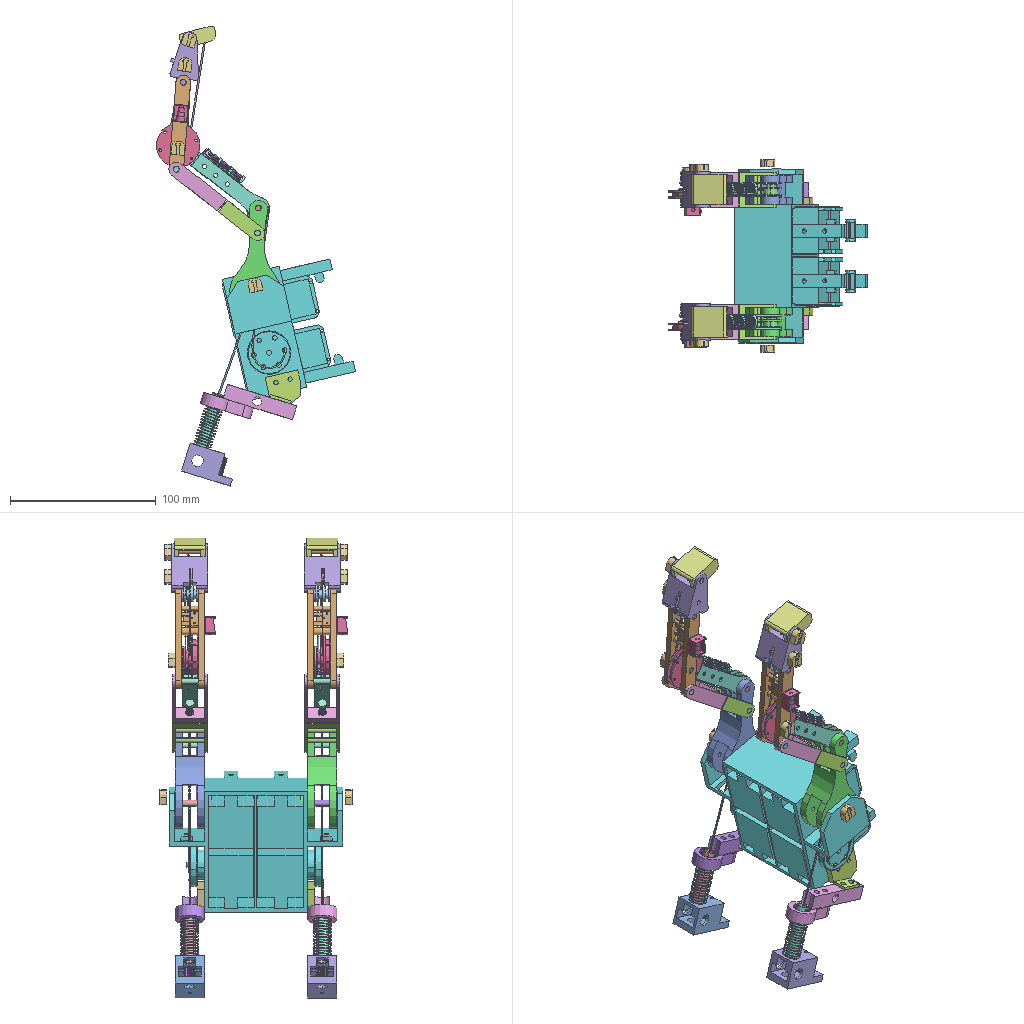Assembly | SolidWorks | 30 different items | 53 placed | box 137 x 132 x 316 mm
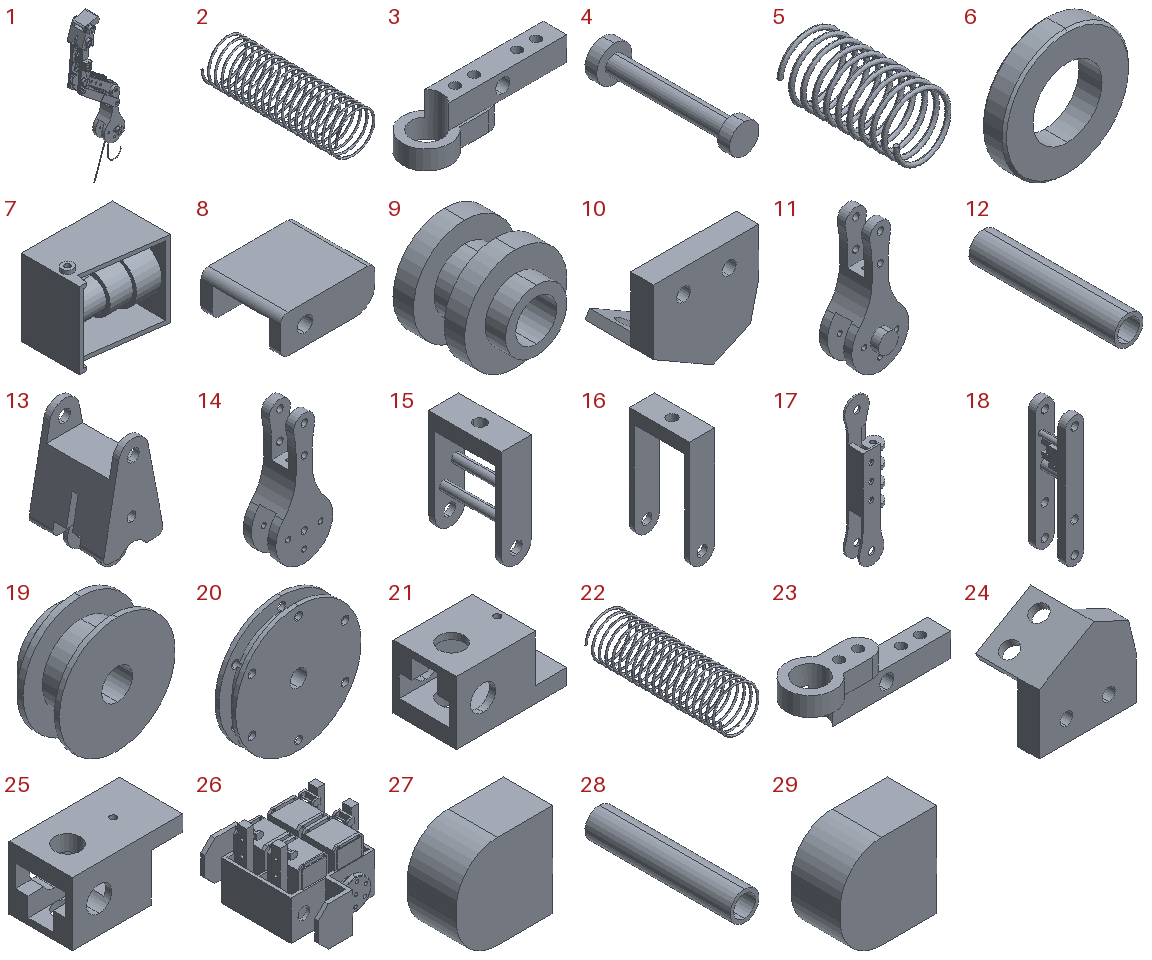Parts list (item | name | quantity | parent item | size | volume | features):
1 | (subassembly) | x1 | - | 88.567 x 35.49 x 253.176 mm | 52231 mm3 | features ReferencePattern 4, CompositeCurve 2, Cut 1, MirrorCompFeat 1
2 | - | x1 | - | 12.5 x 39.277 x 12.5 mm | 146.671 mm3 | features ICE 1, Sweep 1
3 | - | x1 | - | 64 x 20 x 18 mm | 6760 mm3 | features ICE 6, Extrusion 1
4 | - | x2 | in 1 | 6 x 24 x 6 mm | 237.19 mm3 | features Revolution 1
5 | - | x2 | in 1 | 4.3 x 8.352 x 4.3 mm | 8.864 mm3 | features Sweep 1
6 | - | x2 | in 1 | 5.5 x 1 x 5.5 mm | 16.519 mm3 | features Chamfer 1, Extrusion 1
7 | - | x2 | in 1 | 11.794 x 7.578 x 10.5 mm | 389.974 mm3 | features ICE 8, Extrusion 1, Shell 1
8 | - | x2 | in 1 | 25 x 21 x 10 mm | 2190 mm3 | features ICE 4, Fillet 2, Extrusion 1
9 | - | x2 | in 1 | 10 x 9 x 10 mm | 342.434 mm3 | features Extrusion 1, ICE 1, RevCut 1
10 | - | x1 | - | 23 x 15 x 21.606 mm | 2270 mm3 | features ICE 3, Extrusion 1
11 | - | x1 | - | 35 x 25 x 79.915 mm | 17778 mm3 | features ICE 7, Extrusion 1
12 | - | x1 | - | 8 x 40 x 8 mm | 879.646 mm3 | features MirrorStock 1
13 | - | x2 | in 1 | 19.826 x 25 x 40 mm | 7993 mm3 | features ICE 6, Fillet 2, Cut 1, Extrusion 1
14 | - | x1 | in 1 | 35 x 25 x 79.915 mm | 17778 mm3 | features ICE 7, Extrusion 1
15 | - | x2 | in 1 | 10 x 24 x 35 mm | 2527 mm3 | features ICE 4, Extrusion 1
16 | - | x2 | in 1 | 10 x 24 x 45 mm | 2644 mm3 | features ICE 3, Extrusion 1
17 | - | x2 | in 1 | 18.5 x 10 x 85 mm | 2855 mm3 | features ICE 10, Extrusion 1
18 | - | x2 | in 1 | 10 x 20 x 70 mm | 6098 mm3 | features ICE 9, Extrusion 1
19 | - | x2 | in 1 | 15 x 8 x 15 mm | 589.716 mm3 | features ICE 4, RevCut 2, Extrusion 1
20 | - | x2 | in 1 | 30 x 10 x 30 mm | 3231 mm3 | features ICE 3, RevCut 2, Extrusion 1
21 | - | x1 | - | 35 x 20 x 20 mm | 6348 mm3 | features ICE 3, Extrusion 1
22 | - | x1 | - | 12.5 x 39.277 x 12.5 mm | 146.671 mm3 | features MirrorStock 1
23 | - | x1 | - | 64 x 20 x 18 mm | 6760 mm3 | features MirrorStock 1
24 | - | x1 | - | 23 x 15 x 21.606 mm | 2270 mm3 | features MirrorStock 1
25 | - | x1 | - | 35 x 20 x 20 mm | 6348 mm3 | features MirrorStock 1
26 | - | x1 | - | 88.291 x 119.549 x 76 mm | 304358 mm3 | features ICE 21, MirrorPattern 6, Fillet 5, CutThin 3, Chamfer 2, MirrorSolid 2, BossThin 1, DeleteBody 1, ExtruThin 1
27 | - | x8 | in 1 | 9.42 x 4.8 x 9.122 mm | 371.243 mm3 | features MBimport 1, Scale 1
28 | - | x1 | - | 8 x 40 x 8 mm | 879.646 mm3 | features Extrusion 1
29 | - | x4 | in 1 | 9.42 x 4.8 x 9.122 mm | 371.243 mm3 | features MirrorStock 1
30 | spur gear_gb | x1 | - | - | - | -
Mates (type | each side: item.copy, entity, surface, feature):
In the top assembly
Coincident | 11.1 face plane Cut-Extrude4 | 17.1 face plane Boss-Extrude1
Concentric | 11.1 face cylinder Cut-Extrude1 | 17.1 face cylinder Cut-Extrude1
Concentric | 11.1 face cylinder Cut-Extrude1 | 15.1 face cylinder Cut-Extrude2 | 2 times
Coincident | 18.1 face plane Cut-Extrude2 | 13.1 face plane Cut-Extrude2
Parallel | 17.1 face plane Boss-Extrude1 | 18.1 face plane Cut-Extrude2
Concentric | 17.1 face cylinder Cut-Extrude1 | 18.1 face cylinder Cut-Extrude1
Concentric | 18.1 face cylinder Cut-Extrude3 | 13.1 face cylinder Cut-Extrude1
Coincident | 15.1 face plane Boss-Extrude1 | 16.1 face plane Boss-Extrude1
Coincident | 16.1 face plane Cut-Extrude2 | 18.1 face plane Boss-Extrude1
Concentric | 16.1 face cylinder Cut-Extrude1 | 18.1 face cylinder Cut-Extrude1
Concentric | 17.1 face cylinder Cut-Extrude1 | 19.1 face cylinder Cut-Extrude1
Coincident | 17.1 face plane Cut-Extrude4 | 19.1 face plane Boss-Extrude1
Coincident | 18.1 edge | 20.1 face cylinder Cut-Extrude1
Coincident | 18.1 face plane Cut-Extrude2 | 20.1 face plane Boss-Extrude1
Coincident | 13.1 face plane Cut-Extrude4 | 9.1 face plane Boss-Extrude1
Concentric | 18.1 face cylinder Cut-Extrude3 | 9.1 face cylinder Cut-Extrude1
Coincident | 13.1 face plane Cut-Extrude4 | 8.1 face plane Boss-Extrude1
Concentric | 13.1 face cylinder Cut-Extrude1 | 8.1 face cylinder Cut-Extrude3
LimitDistanceDim | 15.1 face plane Boss-Extrude1 | 16.1 face plane Boss-Extrude1
Coincident | 15.1 face plane Cut-Extrude3 | 4.1 face plane Revolve1
Concentric | 15.1 face cylinder Cut-Extrude4 | 4.1 face cylinder Revolve1
Concentric | 16.1 face cylinder Cut-Extrude3 | 4.1 face cylinder Revolve1
Coincident | 4.1 axis | 5.1 select_type:24
Concentric | 16.1 face cylinder Cut-Extrude3 | 6.1 face cylinder Boss-Extrude1
Coincident | 16.1 face plane Cut-Extrude2 | 6.1 face plane Boss-Extrude1
Concentric | 11.1 face cylinder Boss-Extrude2 | 26.1 face cylinder Cut-Extrude1 | 2 times
Coincident | 11.1 face plane Boss-Extrude1 | 26.1 face plane Extrude-Thin1
Coincident | 11.1 face plane Boss-Extrude1 | 15.1 face plane Cut-Extrude3
Concentric | 26.1 face cylinder Cut-Extrude9 | 10.1 face cylinder Cut-Extrude2 | 2 times
Coincident | 26.1 face plane Extrude-Thin1 | 10.1 face plane Boss-Extrude1
Concentric | 10.1 face cylinder Cut-Extrude1 | 3.1 face cylinder Cut-Extrude2 | 2 times
Coincident | 10.1 face plane Boss-Extrude1 | 3.1 face plane Boss-Extrude1
Concentric | 2.1 select_type:24 | 28.1 face cylinder Boss-Extrude1
Parallel | 3.1 face plane Boss-Extrude1 | 21.1 face plane Boss-Extrude1 | 2 times
Concentric | 28.1 face cylinder Boss-Extrude1 | 21.1 face cylinder Cut-Extrude1 | 2 times
Concentric | 3.1 face cylinder Cut-Extrude6 | 28.1 face cylinder Boss-Extrude1
LimitDistanceDim | 28.1 face plane Boss-Extrude1 | 3.1 face plane Boss-Extrude2
Coincident | 28.1 face plane Boss-Extrude1 | 21.1 face plane Cut-Extrude4
Lock | 4.1 select_type:0 | 5.1 select_type:0
InPlace | 18.1 face plane Boss-Extrude1 | 7.1 plane
Coincident | 18.1 face plane Boss-Extrude1 | 27.1 face plane Sensor.STEP<1>
Coincident | 13.1 face plane Boss-Extrude1 | 27.2 face plane Sensor.STEP<1>
Coincident | 13.1 face plane Boss-Extrude1 | 27.3 face plane Sensor.STEP<1>
Concentric | 26.1 face cylinder Cut-Extrude1 | 14.1 face cylinder Boss-Extrude2
Coincident | 26.1 face plane Extrude-Thin1 | 14.1 face plane Boss-Extrude1
In subassembly 1
Coincident | 14.2 face plane Cut-Extrude4 | 17.1 face plane Boss-Extrude1
Concentric | 14.2 face cylinder Cut-Extrude1 | 17.1 face cylinder Cut-Extrude1
Concentric | 14.2 face cylinder Cut-Extrude1 | 15.1 face cylinder Cut-Extrude2 | 2 times
Coincident | 18.1 face plane Cut-Extrude2 | 13.1 face plane Cut-Extrude2
Parallel | 17.1 face plane Boss-Extrude1 | 18.1 face plane Cut-Extrude2
Concentric | 17.1 face cylinder Cut-Extrude1 | 18.1 face cylinder Cut-Extrude1
Concentric | 18.1 face cylinder Cut-Extrude3 | 13.1 face cylinder Cut-Extrude1
Coincident | 15.1 face plane Boss-Extrude1 | 16.1 face plane Boss-Extrude1
Coincident | 16.1 face plane Cut-Extrude2 | 18.1 face plane Boss-Extrude1
Concentric | 16.1 face cylinder Cut-Extrude1 | 18.1 face cylinder Cut-Extrude1
Concentric | 17.1 face cylinder Cut-Extrude1 | 19.1 face cylinder Cut-Extrude1
Coincident | 17.1 face plane Cut-Extrude4 | 19.1 face plane Boss-Extrude1
Coincident | 18.1 edge | 20.1 face cylinder Cut-Extrude1
Coincident | 18.1 face plane Cut-Extrude2 | 20.1 face plane Boss-Extrude1
Coincident | 13.1 face plane Cut-Extrude4 | 9.1 face plane Boss-Extrude1
Concentric | 18.1 face cylinder Cut-Extrude3 | 9.1 face cylinder Cut-Extrude1
Coincident | 13.1 face plane Cut-Extrude4 | 8.1 face plane Boss-Extrude1
Concentric | 13.1 face cylinder Cut-Extrude1 | 8.1 face cylinder Cut-Extrude3
LimitDistanceDim | 15.1 face plane Boss-Extrude1 | 16.1 face plane Boss-Extrude1
Coincident | 15.1 face plane Cut-Extrude3 | 4.1 face plane Revolve1
Concentric | 15.1 face cylinder Cut-Extrude4 | 4.1 face cylinder Revolve1
Concentric | 16.1 face cylinder Cut-Extrude3 | 4.1 face cylinder Revolve1
Coincident | 4.1 axis | 5.1 select_type:24
Concentric | 16.1 face cylinder Cut-Extrude3 | 6.1 face cylinder Boss-Extrude1
Coincident | 16.1 face plane Cut-Extrude2 | 6.1 face plane Boss-Extrude1
Coincident | 14.2 face plane Boss-Extrude1 | 15.1 face plane Cut-Extrude3
Lock | 4.1 select_type:0 | 5.1 select_type:0
InPlace | 18.1 face plane Boss-Extrude1 | 7.1 plane
Coincident | 18.1 face plane Boss-Extrude1 | 27.1 face plane Sensor.STEP<1>
Coincident | 13.1 face plane Boss-Extrude1 | 27.2 face plane Sensor.STEP<1>
Coincident | 13.1 face plane Boss-Extrude1 | 27.3 face plane Sensor.STEP<1>